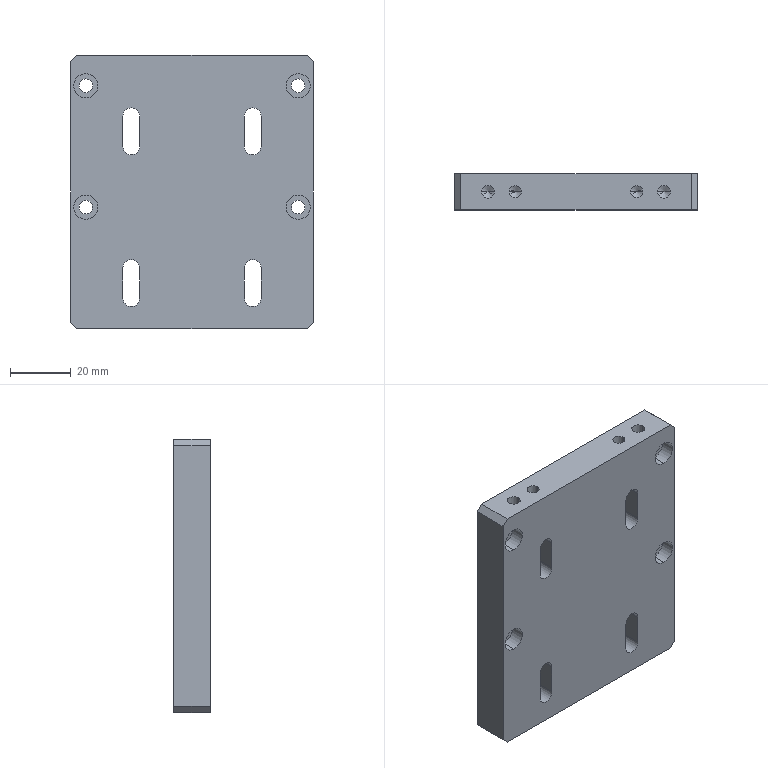Part | STEP file | PN_0032 | 1 solid | 66 faces | box 80 x 12 x 90 mm | volume 80517 mm3 | cylinder 36 | plane 22 | cone 8 | commonest cylinder face diameters 5.5 x12 4.5 x8 8 x8 4 x4 4.2 x4